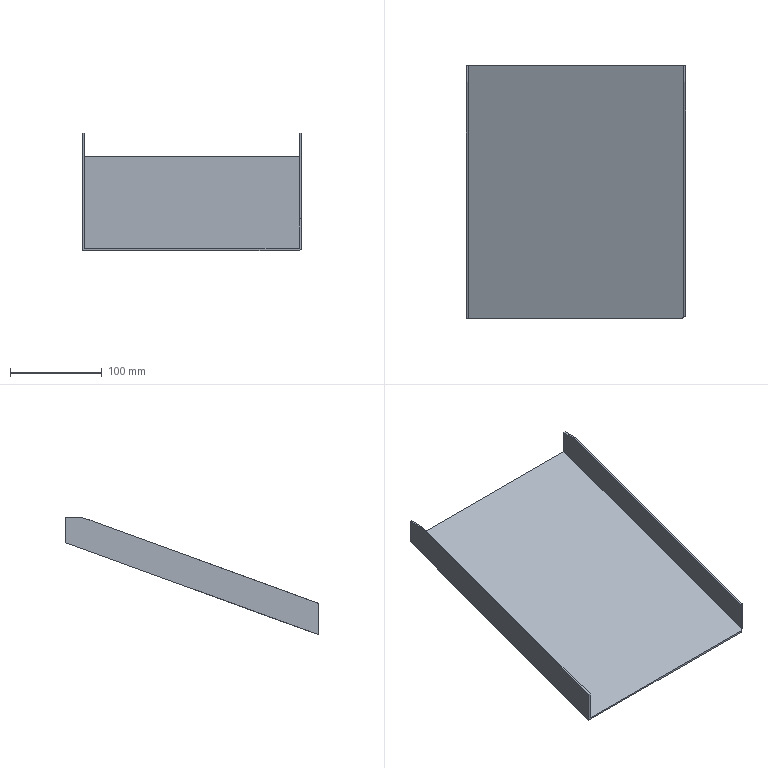Part | NX | features HB 2 | 1 solid | 13 faces | box 239 x 275.381 x 127.795 mm | volume 174868 mm3 | plane 12 | cylinder 1 | commonest cylinder face diameters 190 x1
STEP:
#1=CARTESIAN_POINT('',(590.54,382.551,-213.));
#2=VERTEX_POINT('',#1);
#3=CARTESIAN_POINT('',(590.54,400.381,-213.));
#4=VERTEX_POINT('',#3);
#5=CARTESIAN_POINT('',(590.54,20.77,-213.));
#6=DIRECTION('',(0.,1.,0.));
#7=VECTOR('',#6,1000.);
#8=LINE('',#5,#7);
#9=EDGE_CURVE('',#2,#4,#8,.T.);
#10=ORIENTED_EDGE('',*,*,#9,.F.);
#11=CARTESIAN_POINT('',(590.54,127.84,-305.707));
#12=VERTEX_POINT('',#11);
#13=CARTESIAN_POINT('',(590.54,10.51,-348.412));
#14=DIRECTION('',(0.,0.9397,0.342));
#15=VECTOR('',#14,1000.);
#16=LINE('',#13,#15);
#17=EDGE_CURVE('',#12,#2,#16,.T.);
#18=ORIENTED_EDGE('',*,*,#17,.F.);
#19=CARTESIAN_POINT('',(590.54,127.84,-339.761));
#20=VERTEX_POINT('',#19);
#21=CARTESIAN_POINT('',(590.54,127.84,-305.707));
#22=DIRECTION('',(0.,0.,-1.));
#23=VECTOR('',#22,1000.);
#24=LINE('',#21,#23);
#25=EDGE_CURVE('',#12,#20,#24,.T.);
#26=ORIENTED_EDGE('',*,*,#25,.T.);
#27=CARTESIAN_POINT('',(590.54,400.381,-240.564));
#28=VERTEX_POINT('',#27);
#29=CARTESIAN_POINT('',(590.54,21.454,-378.482));
#30=DIRECTION('',(0.,-0.9397,-0.342));
#31=VECTOR('',#30,1000.);
#32=LINE('',#29,#31);
#33=EDGE_CURVE('',#28,#20,#32,.T.);
#34=ORIENTED_EDGE('',*,*,#33,.F.);
#35=CARTESIAN_POINT('',(590.54,400.381,-376.603));
#36=DIRECTION('',(0.,0.,1.));
#37=VECTOR('',#36,1000.);
#38=LINE('',#35,#37);
#39=EDGE_CURVE('',#28,#4,#38,.T.);
#40=ORIENTED_EDGE('',*,*,#39,.T.);
#41=EDGE_LOOP('',(#10,#18,#26,#34,#40));
#42=FACE_BOUND('',#41,.T.);
#43=CARTESIAN_POINT('',(590.54,20.77,-376.603));
#44=DIRECTION('',(-1.,0.,0.));
#45=DIRECTION('',(0.,-0.08716,-0.9962));
#46=AXIS2_PLACEMENT_3D('',#43,#44,#45);
#47=PLANE('',#46);
#48=ADVANCED_FACE('',(#42),#47,.F.);
#49=CARTESIAN_POINT('',(588.54,126.402,-306.231));
#50=VERTEX_POINT('',#49);
#51=CARTESIAN_POINT('',(588.54,382.551,-213.));
#52=VERTEX_POINT('',#51);
#53=CARTESIAN_POINT('',(588.54,10.51,-348.412));
#54=DIRECTION('',(0.,0.9397,0.342));
#55=VECTOR('',#54,1000.);
#56=LINE('',#53,#55);
#57=EDGE_CURVE('',#50,#52,#56,.T.);
#58=ORIENTED_EDGE('',*,*,#57,.T.);
#59=CARTESIAN_POINT('',(588.54,400.381,-213.));
#60=VERTEX_POINT('',#59);
#61=CARTESIAN_POINT('',(588.54,20.77,-213.));
#62=DIRECTION('',(0.,1.,0.));
#63=VECTOR('',#62,1000.);
#64=LINE('',#61,#63);
#65=EDGE_CURVE('',#52,#60,#64,.T.);
#66=ORIENTED_EDGE('',*,*,#65,.T.);
#67=CARTESIAN_POINT('',(588.54,400.381,-238.436));
#68=VERTEX_POINT('',#67);
#69=CARTESIAN_POINT('',(588.54,400.381,-376.603));
#70=DIRECTION('',(0.,0.,1.));
#71=VECTOR('',#70,1000.);
#72=LINE('',#69,#71);
#73=EDGE_CURVE('',#68,#60,#72,.T.);
#74=ORIENTED_EDGE('',*,*,#73,.F.);
#75=CARTESIAN_POINT('',(588.54,126.402,-338.156));
#76=VERTEX_POINT('',#75);
#77=CARTESIAN_POINT('',(588.54,20.77,-376.603));
#78=DIRECTION('',(0.,0.9397,0.342));
#79=VECTOR('',#78,1000.);
#80=LINE('',#77,#79);
#81=EDGE_CURVE('',#76,#68,#80,.T.);
#82=ORIENTED_EDGE('',*,*,#81,.F.);
#83=CARTESIAN_POINT('',(588.54,126.402,-338.156));
#84=DIRECTION('',(0.,0.,1.));
#85=VECTOR('',#84,1000.);
#86=LINE('',#83,#85);
#87=EDGE_CURVE('',#76,#50,#86,.T.);
#88=ORIENTED_EDGE('',*,*,#87,.T.);
#89=EDGE_LOOP('',(#58,#66,#74,#82,#88));
#90=FACE_BOUND('',#89,.T.);
#91=CARTESIAN_POINT('',(588.54,20.77,-376.603));
#92=DIRECTION('',(-1.,0.,0.));
#93=DIRECTION('',(0.,0.08716,0.9962));
#94=AXIS2_PLACEMENT_3D('',#91,#92,#93);
#95=PLANE('',#94);
#96=ADVANCED_FACE('',(#90),#95,.T.);
#97=CARTESIAN_POINT('',(698.54,382.551,-213.));
#98=DIRECTION('',(1.,0.,0.));
#99=VECTOR('',#98,1000.);
#100=LINE('',#97,#99);
#101=EDGE_CURVE('',#52,#2,#100,.T.);
#102=ORIENTED_EDGE('',*,*,#101,.F.);
#103=ORIENTED_EDGE('',*,*,#57,.F.);
#104=CARTESIAN_POINT('',(645.,50.,-334.039));
#105=DIRECTION('',(0.,0.342,-0.9397));
#106=DIRECTION('',(0.,0.9397,0.342));
#107=AXIS2_PLACEMENT_3D('',#104,#105,#106);
#108=ELLIPSE('',#107,101.097,95.);
#109=EDGE_CURVE('',#50,#12,#108,.T.);
#110=ORIENTED_EDGE('',*,*,#109,.T.);
#111=ORIENTED_EDGE('',*,*,#17,.T.);
#112=EDGE_LOOP('',(#102,#103,#110,#111));
#113=FACE_BOUND('',#112,.T.);
#114=CARTESIAN_POINT('',(698.54,10.51,-348.412));
#115=DIRECTION('',(0.,0.342,-0.9397));
#116=DIRECTION('',(0.,-0.9397,-0.342));
#117=AXIS2_PLACEMENT_3D('',#114,#115,#116);
#118=PLANE('',#117);
#119=ADVANCED_FACE('',(#113),#118,.F.);
#120=CARTESIAN_POINT('',(351.54,400.381,-213.));
#121=VERTEX_POINT('',#120);
#122=CARTESIAN_POINT('',(351.54,382.551,-213.));
#123=VERTEX_POINT('',#122);
#124=CARTESIAN_POINT('',(351.54,20.77,-213.));
#125=DIRECTION('',(0.,-1.,0.));
#126=VECTOR('',#125,1000.);
#127=LINE('',#124,#126);
#128=EDGE_CURVE('',#121,#123,#127,.T.);
#129=ORIENTED_EDGE('',*,*,#128,.F.);
#130=CARTESIAN_POINT('',(351.54,400.381,-240.564));
#131=VERTEX_POINT('',#130);
#132=CARTESIAN_POINT('',(351.54,400.381,-376.603));
#133=DIRECTION('',(0.,0.,-1.));
#134=VECTOR('',#133,1000.);
#135=LINE('',#132,#134);
#136=EDGE_CURVE('',#121,#131,#135,.T.);
#137=ORIENTED_EDGE('',*,*,#136,.T.);
#138=CARTESIAN_POINT('',(351.54,125.,-340.795));
#139=VERTEX_POINT('',#138);
#140=CARTESIAN_POINT('',(351.54,21.454,-378.482));
#141=DIRECTION('',(0.,0.9397,0.342));
#142=VECTOR('',#141,1000.);
#143=LINE('',#140,#142);
#144=EDGE_CURVE('',#139,#131,#143,.T.);
#145=ORIENTED_EDGE('',*,*,#144,.F.);
#146=CARTESIAN_POINT('',(351.54,125.,-306.741));
#147=VERTEX_POINT('',#146);
#148=CARTESIAN_POINT('',(351.54,125.,-376.603));
#149=DIRECTION('',(0.,0.,-1.));
#150=VECTOR('',#149,1000.);
#151=LINE('',#148,#150);
#152=EDGE_CURVE('',#147,#139,#151,.T.);
#153=ORIENTED_EDGE('',*,*,#152,.F.);
#154=CARTESIAN_POINT('',(351.54,10.51,-348.412));
#155=DIRECTION('',(0.,0.9397,0.342));
#156=VECTOR('',#155,1000.);
#157=LINE('',#154,#156);
#158=EDGE_CURVE('',#147,#123,#157,.T.);
#159=ORIENTED_EDGE('',*,*,#158,.T.);
#160=EDGE_LOOP('',(#129,#137,#145,#153,#159));
#161=FACE_BOUND('',#160,.T.);
#162=CARTESIAN_POINT('',(351.54,20.77,-376.603));
#163=DIRECTION('',(1.,0.,0.));
#164=DIRECTION('',(0.,0.08716,0.9962));
#165=AXIS2_PLACEMENT_3D('',#162,#163,#164);
#166=PLANE('',#165);
#167=ADVANCED_FACE('',(#161),#166,.F.);
#168=CARTESIAN_POINT('',(353.54,400.381,-213.));
#169=VERTEX_POINT('',#168);
#170=CARTESIAN_POINT('',(353.54,400.381,-238.436));
#171=VERTEX_POINT('',#170);
#172=CARTESIAN_POINT('',(353.54,400.381,-376.603));
#173=DIRECTION('',(0.,0.,-1.));
#174=VECTOR('',#173,1000.);
#175=LINE('',#172,#174);
#176=EDGE_CURVE('',#169,#171,#175,.T.);
#177=ORIENTED_EDGE('',*,*,#176,.F.);
#178=CARTESIAN_POINT('',(353.54,382.551,-213.));
#179=VERTEX_POINT('',#178);
#180=CARTESIAN_POINT('',(353.54,20.77,-213.));
#181=DIRECTION('',(0.,-1.,0.));
#182=VECTOR('',#181,1000.);
#183=LINE('',#180,#182);
#184=EDGE_CURVE('',#169,#179,#183,.T.);
#185=ORIENTED_EDGE('',*,*,#184,.T.);
#186=CARTESIAN_POINT('',(353.54,125.,-306.741));
#187=VERTEX_POINT('',#186);
#188=CARTESIAN_POINT('',(353.54,10.51,-348.412));
#189=DIRECTION('',(0.,0.9397,0.342));
#190=VECTOR('',#189,1000.);
#191=LINE('',#188,#190);
#192=EDGE_CURVE('',#187,#179,#191,.T.);
#193=ORIENTED_EDGE('',*,*,#192,.F.);
#194=CARTESIAN_POINT('',(353.54,125.,-338.666));
#195=VERTEX_POINT('',#194);
#196=CARTESIAN_POINT('',(353.54,125.,-376.603));
#197=DIRECTION('',(0.,0.,-1.));
#198=VECTOR('',#197,1000.);
#199=LINE('',#196,#198);
#200=EDGE_CURVE('',#187,#195,#199,.T.);
#201=ORIENTED_EDGE('',*,*,#200,.T.);
#202=CARTESIAN_POINT('',(353.54,20.77,-376.603));
#203=DIRECTION('',(0.,-0.9397,-0.342));
#204=VECTOR('',#203,1000.);
#205=LINE('',#202,#204);
#206=EDGE_CURVE('',#171,#195,#205,.T.);
#207=ORIENTED_EDGE('',*,*,#206,.F.);
#208=EDGE_LOOP('',(#177,#185,#193,#201,#207));
#209=FACE_BOUND('',#208,.T.);
#210=CARTESIAN_POINT('',(353.54,20.77,-376.603));
#211=DIRECTION('',(1.,0.,0.));
#212=DIRECTION('',(0.,0.08716,0.9962));
#213=AXIS2_PLACEMENT_3D('',#210,#211,#212);
#214=PLANE('',#213);
#215=ADVANCED_FACE('',(#209),#214,.T.);
#216=CARTESIAN_POINT('',(376.54,382.551,-213.));
#217=DIRECTION('',(1.,0.,0.));
#218=VECTOR('',#217,1000.);
#219=LINE('',#216,#218);
#220=EDGE_CURVE('',#123,#179,#219,.T.);
#221=ORIENTED_EDGE('',*,*,#220,.F.);
#222=ORIENTED_EDGE('',*,*,#158,.F.);
#223=CARTESIAN_POINT('',(376.54,125.,-306.741));
#224=DIRECTION('',(-1.,0.,0.));
#225=VECTOR('',#224,1000.);
#226=LINE('',#223,#225);
#227=EDGE_CURVE('',#187,#147,#226,.T.);
#228=ORIENTED_EDGE('',*,*,#227,.F.);
#229=ORIENTED_EDGE('',*,*,#192,.T.);
#230=EDGE_LOOP('',(#221,#222,#228,#229));
#231=FACE_BOUND('',#230,.T.);
#232=CARTESIAN_POINT('',(376.54,10.51,-348.412));
#233=DIRECTION('',(0.,0.342,-0.9397));
#234=DIRECTION('',(0.,-0.9397,-0.342));
#235=AXIS2_PLACEMENT_3D('',#232,#233,#234);
#236=PLANE('',#235);
#237=ADVANCED_FACE('',(#231),#236,.F.);
#238=ORIENTED_EDGE('',*,*,#136,.F.);
#239=CARTESIAN_POINT('',(99.54,400.381,-213.));
#240=DIRECTION('',(1.,0.,0.));
#241=VECTOR('',#240,1000.);
#242=LINE('',#239,#241);
#243=EDGE_CURVE('',#121,#169,#242,.T.);
#244=ORIENTED_EDGE('',*,*,#243,.T.);
#245=ORIENTED_EDGE('',*,*,#176,.T.);
#246=CARTESIAN_POINT('',(608.54,400.381,-238.436));
#247=DIRECTION('',(1.,0.,0.));
#248=VECTOR('',#247,1000.);
#249=LINE('',#246,#248);
#250=EDGE_CURVE('',#171,#68,#249,.T.);
#251=ORIENTED_EDGE('',*,*,#250,.T.);
#252=ORIENTED_EDGE('',*,*,#73,.T.);
#253=CARTESIAN_POINT('',(84.54,400.381,-213.));
#254=DIRECTION('',(1.,0.,0.));
#255=VECTOR('',#254,1000.);
#256=LINE('',#253,#255);
#257=EDGE_CURVE('',#60,#4,#256,.T.);
#258=ORIENTED_EDGE('',*,*,#257,.T.);
#259=ORIENTED_EDGE('',*,*,#39,.F.);
#260=CARTESIAN_POINT('',(608.54,400.381,-240.564));
#261=DIRECTION('',(1.,0.,0.));
#262=VECTOR('',#261,1000.);
#263=LINE('',#260,#262);
#264=EDGE_CURVE('',#131,#28,#263,.T.);
#265=ORIENTED_EDGE('',*,*,#264,.F.);
#266=EDGE_LOOP('',(#238,#244,#245,#251,#252,#258,#259,#265));
#267=FACE_BOUND('',#266,.T.);
#268=CARTESIAN_POINT('',(99.54,400.381,0.));
#269=DIRECTION('',(0.,1.,0.));
#270=DIRECTION('',(0.,0.,-1.));
#271=AXIS2_PLACEMENT_3D('',#268,#269,#270);
#272=PLANE('',#271);
#273=ADVANCED_FACE('',(#267),#272,.T.);
#274=CARTESIAN_POINT('',(586.69,125.,-340.795));
#275=VERTEX_POINT('',#274);
#276=CARTESIAN_POINT('',(608.54,125.,-340.795));
#277=DIRECTION('',(1.,0.,0.));
#278=VECTOR('',#277,1000.);
#279=LINE('',#276,#278);
#280=EDGE_CURVE('',#139,#275,#279,.T.);
#281=ORIENTED_EDGE('',*,*,#280,.T.);
#282=CARTESIAN_POINT('',(586.69,125.,-338.666));
#283=VERTEX_POINT('',#282);
#284=CARTESIAN_POINT('',(586.69,125.,-1480.5));
#285=DIRECTION('',(0.,0.,1.));
#286=VECTOR('',#285,1000.);
#287=LINE('',#284,#286);
#288=EDGE_CURVE('',#275,#283,#287,.T.);
#289=ORIENTED_EDGE('',*,*,#288,.T.);
#290=CARTESIAN_POINT('',(608.54,125.,-338.666));
#291=DIRECTION('',(1.,0.,0.));
#292=VECTOR('',#291,1000.);
#293=LINE('',#290,#292);
#294=EDGE_CURVE('',#195,#283,#293,.T.);
#295=ORIENTED_EDGE('',*,*,#294,.F.);
#296=ORIENTED_EDGE('',*,*,#200,.F.);
#297=ORIENTED_EDGE('',*,*,#227,.T.);
#298=ORIENTED_EDGE('',*,*,#152,.T.);
#299=EDGE_LOOP('',(#281,#289,#295,#296,#297,#298));
#300=FACE_BOUND('',#299,.T.);
#301=CARTESIAN_POINT('',(845.,125.,-2230.5));
#302=DIRECTION('',(0.,1.,0.));
#303=DIRECTION('',(0.,0.,-1.));
#304=AXIS2_PLACEMENT_3D('',#301,#302,#303);
#305=PLANE('',#304);
#306=ADVANCED_FACE('',(#300),#305,.F.);
#307=ORIENTED_EDGE('',*,*,#294,.T.);
#308=CARTESIAN_POINT('',(645.,50.,-365.964));
#309=DIRECTION('',(0.,-0.342,0.9397));
#310=DIRECTION('',(0.,0.9397,0.342));
#311=AXIS2_PLACEMENT_3D('',#308,#309,#310);
#312=ELLIPSE('',#311,101.097,95.);
#313=EDGE_CURVE('',#76,#283,#312,.T.);
#314=ORIENTED_EDGE('',*,*,#313,.F.);
#315=ORIENTED_EDGE('',*,*,#81,.T.);
#316=ORIENTED_EDGE('',*,*,#250,.F.);
#317=ORIENTED_EDGE('',*,*,#206,.T.);
#318=EDGE_LOOP('',(#307,#314,#315,#316,#317));
#319=FACE_BOUND('',#318,.T.);
#320=CARTESIAN_POINT('',(608.54,20.77,-376.603));
#321=DIRECTION('',(0.,-0.342,0.9397));
#322=DIRECTION('',(-1.,0.,0.));
#323=AXIS2_PLACEMENT_3D('',#320,#321,#322);
#324=PLANE('',#323);
#325=ADVANCED_FACE('',(#319),#324,.T.);
#326=CARTESIAN_POINT('',(645.,50.,-368.092));
#327=DIRECTION('',(0.,-0.342,0.9397));
#328=DIRECTION('',(0.,0.9397,0.342));
#329=AXIS2_PLACEMENT_3D('',#326,#327,#328);
#330=ELLIPSE('',#329,101.097,95.);
#331=EDGE_CURVE('',#20,#275,#330,.T.);
#332=ORIENTED_EDGE('',*,*,#331,.T.);
#333=ORIENTED_EDGE('',*,*,#280,.F.);
#334=ORIENTED_EDGE('',*,*,#144,.T.);
#335=ORIENTED_EDGE('',*,*,#264,.T.);
#336=ORIENTED_EDGE('',*,*,#33,.T.);
#337=EDGE_LOOP('',(#332,#333,#334,#335,#336));
#338=FACE_BOUND('',#337,.T.);
#339=CARTESIAN_POINT('',(608.54,21.454,-378.482));
#340=DIRECTION('',(0.,-0.342,0.9397));
#341=DIRECTION('',(-1.,0.,0.));
#342=AXIS2_PLACEMENT_3D('',#339,#340,#341);
#343=PLANE('',#342);
#344=ADVANCED_FACE('',(#338),#343,.F.);
#345=ORIENTED_EDGE('',*,*,#87,.F.);
#346=ORIENTED_EDGE('',*,*,#313,.T.);
#347=ORIENTED_EDGE('',*,*,#288,.F.);
#348=ORIENTED_EDGE('',*,*,#331,.F.);
#349=ORIENTED_EDGE('',*,*,#25,.F.);
#350=ORIENTED_EDGE('',*,*,#109,.F.);
#351=EDGE_LOOP('',(#345,#346,#347,#348,#349,#350));
#352=FACE_BOUND('',#351,.T.);
#353=CARTESIAN_POINT('',(645.,50.,-1480.5));
#354=DIRECTION('',(0.,0.,1.));
#355=DIRECTION('',(-1.,0.,0.));
#356=AXIS2_PLACEMENT_3D('',#353,#354,#355);
#357=CYLINDRICAL_SURFACE('',#356,95.);
#358=ADVANCED_FACE('',(#352),#357,.F.);
#359=ORIENTED_EDGE('',*,*,#65,.F.);
#360=ORIENTED_EDGE('',*,*,#101,.T.);
#361=ORIENTED_EDGE('',*,*,#9,.T.);
#362=ORIENTED_EDGE('',*,*,#257,.F.);
#363=EDGE_LOOP('',(#359,#360,#361,#362));
#364=FACE_BOUND('',#363,.T.);
#365=CARTESIAN_POINT('',(1930.,0.,-213.));
#366=DIRECTION('',(0.,0.,1.));
#367=DIRECTION('',(-1.,0.,0.));
#368=AXIS2_PLACEMENT_3D('',#365,#366,#367);
#369=PLANE('',#368);
#370=ADVANCED_FACE('',(#364),#369,.T.);
#371=ORIENTED_EDGE('',*,*,#128,.T.);
#372=ORIENTED_EDGE('',*,*,#220,.T.);
#373=ORIENTED_EDGE('',*,*,#184,.F.);
#374=ORIENTED_EDGE('',*,*,#243,.F.);
#375=EDGE_LOOP('',(#371,#372,#373,#374));
#376=FACE_BOUND('',#375,.T.);
#377=CARTESIAN_POINT('',(1945.,0.,-213.));
#378=DIRECTION('',(0.,0.,1.));
#379=DIRECTION('',(-1.,0.,0.));
#380=AXIS2_PLACEMENT_3D('',#377,#378,#379);
#381=PLANE('',#380);
#382=ADVANCED_FACE('',(#376),#381,.T.);
#383=CLOSED_SHELL('',(#48,#96,#119,#167,#215,#237,#273,#306,#325,#344,#358,#370,#382));
#384=MANIFOLD_SOLID_BREP('',#383);
#385=(LENGTH_UNIT()NAMED_UNIT(*)SI_UNIT(.MILLI.,.METRE.));
#386=UNCERTAINTY_MEASURE_WITH_UNIT(LENGTH_MEASURE(0.00001),#385,'','');
#387=(NAMED_UNIT(*)PLANE_ANGLE_UNIT()SI_UNIT($,.RADIAN.));
#388=(NAMED_UNIT(*)SI_UNIT($,.STERADIAN.)SOLID_ANGLE_UNIT());
#389=(GEOMETRIC_REPRESENTATION_CONTEXT(3)GLOBAL_UNCERTAINTY_ASSIGNED_CONTEXT((#386))GLOBAL_UNIT_ASSIGNED_CONTEXT((#385,#387,#388))REPRESENTATION_CONTEXT('',''));
#390=ADVANCED_BREP_SHAPE_REPRESENTATION('',(#384),#389);